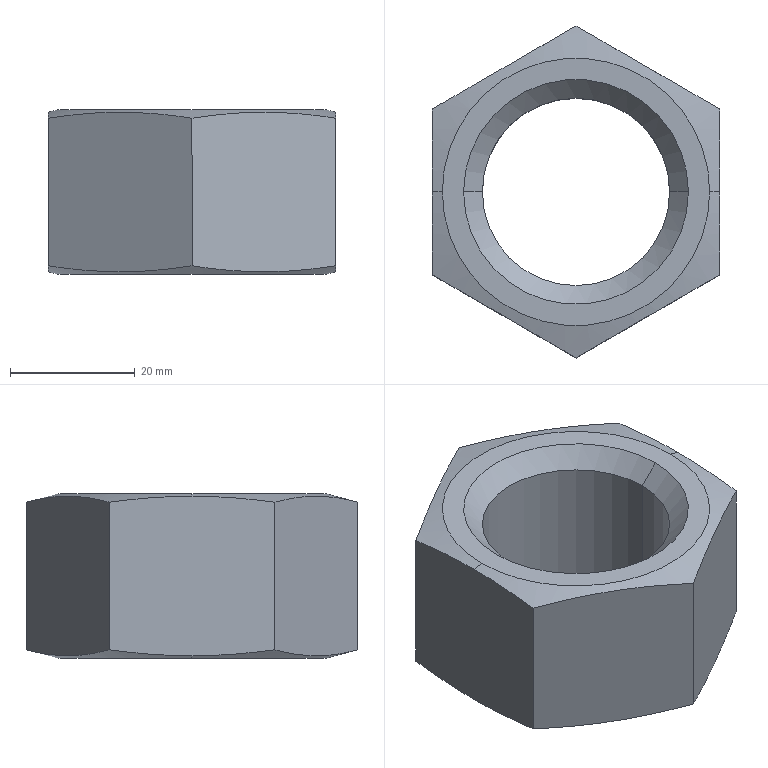Part | SolidWorks | features Chamfer 1, Extrusion 1, ICE 1, MirrorPattern 1, RevCutThin 1 | 1 solid | 18 faces | box 46 x 53.116 x 26.4 mm | volume 28471 mm3 | cone 8 | plane 8 | cylinder 2 | commonest cylinder face diameters 30 x2
STEP:
#1=CARTESIAN_POINT('',(-15.,0.,10.2));
#2=VERTEX_POINT('',#1);
#3=CARTESIAN_POINT('',(15.,0.,10.2));
#4=VERTEX_POINT('',#3);
#5=CARTESIAN_POINT('',(0.,0.,10.2));
#6=DIRECTION('',(0.,0.,1.));
#7=DIRECTION('',(1.,0.,0.));
#8=AXIS2_PLACEMENT_3D('',#5,#6,#7);
#9=CIRCLE('',#8,15.);
#10=EDGE_CURVE('',#2,#4,#9,.T.);
#11=ORIENTED_EDGE('',*,*,#10,.F.);
#12=CARTESIAN_POINT('',(-18.,0.,13.2));
#13=VERTEX_POINT('',#12);
#14=CARTESIAN_POINT('',(-15.,0.,10.2));
#15=DIRECTION('',(-0.7071,0.,0.7071));
#16=VECTOR('',#15,1000.);
#17=LINE('',#14,#16);
#18=EDGE_CURVE('',#2,#13,#17,.T.);
#19=ORIENTED_EDGE('',*,*,#18,.T.);
#20=CARTESIAN_POINT('',(18.,0.,13.2));
#21=VERTEX_POINT('',#20);
#22=CARTESIAN_POINT('',(0.,0.,13.2));
#23=DIRECTION('',(0.,0.,-1.));
#24=DIRECTION('',(1.,0.,0.));
#25=AXIS2_PLACEMENT_3D('',#22,#23,#24);
#26=CIRCLE('',#25,18.);
#27=EDGE_CURVE('',#21,#13,#26,.T.);
#28=ORIENTED_EDGE('',*,*,#27,.F.);
#29=CARTESIAN_POINT('',(15.,0.,10.2));
#30=DIRECTION('',(0.7071,0.,0.7071));
#31=VECTOR('',#30,1000.);
#32=LINE('',#29,#31);
#33=EDGE_CURVE('',#4,#21,#32,.T.);
#34=ORIENTED_EDGE('',*,*,#33,.F.);
#35=EDGE_LOOP('',(#11,#19,#28,#34));
#36=FACE_OUTER_BOUND('',#35,.T.);
#37=CARTESIAN_POINT('',(0.,0.,10.2));
#38=DIRECTION('',(0.,0.,1.));
#39=DIRECTION('',(1.,0.,0.));
#40=AXIS2_PLACEMENT_3D('',#37,#38,#39);
#41=CONICAL_SURFACE('',#40,15.,0.7854);
#42=ADVANCED_FACE('',(#36),#41,.F.);
#43=CARTESIAN_POINT('',(15.,0.,-10.2));
#44=VERTEX_POINT('',#43);
#45=CARTESIAN_POINT('',(-15.,0.,-10.2));
#46=VERTEX_POINT('',#45);
#47=CARTESIAN_POINT('',(0.,0.,-10.2));
#48=DIRECTION('',(0.,0.,-1.));
#49=DIRECTION('',(1.,0.,0.));
#50=AXIS2_PLACEMENT_3D('',#47,#48,#49);
#51=CIRCLE('',#50,15.);
#52=EDGE_CURVE('',#44,#46,#51,.T.);
#53=ORIENTED_EDGE('',*,*,#52,.F.);
#54=CARTESIAN_POINT('',(18.,0.,-13.2));
#55=VERTEX_POINT('',#54);
#56=CARTESIAN_POINT('',(18.,0.,-13.2));
#57=DIRECTION('',(0.7071,0.,-0.7071));
#58=VECTOR('',#57,1000.);
#59=LINE('',#56,#58);
#60=EDGE_CURVE('',#44,#55,#59,.T.);
#61=ORIENTED_EDGE('',*,*,#60,.T.);
#62=CARTESIAN_POINT('',(-18.,0.,-13.2));
#63=VERTEX_POINT('',#62);
#64=CARTESIAN_POINT('',(0.,0.,-13.2));
#65=DIRECTION('',(0.,0.,1.));
#66=DIRECTION('',(1.,0.,0.));
#67=AXIS2_PLACEMENT_3D('',#64,#65,#66);
#68=CIRCLE('',#67,18.);
#69=EDGE_CURVE('',#63,#55,#68,.T.);
#70=ORIENTED_EDGE('',*,*,#69,.F.);
#71=CARTESIAN_POINT('',(-18.,0.,-13.2));
#72=DIRECTION('',(-0.7071,0.,-0.7071));
#73=VECTOR('',#72,1000.);
#74=LINE('',#71,#73);
#75=EDGE_CURVE('',#46,#63,#74,.T.);
#76=ORIENTED_EDGE('',*,*,#75,.F.);
#77=EDGE_LOOP('',(#53,#61,#70,#76));
#78=FACE_OUTER_BOUND('',#77,.T.);
#79=CARTESIAN_POINT('',(0.,0.,-13.2));
#80=DIRECTION('',(0.,0.,-1.));
#81=DIRECTION('',(-1.,0.,0.));
#82=AXIS2_PLACEMENT_3D('',#79,#80,#81);
#83=CONICAL_SURFACE('',#82,18.,0.7854);
#84=ADVANCED_FACE('',(#78),#83,.F.);
#85=ORIENTED_EDGE('',*,*,#52,.T.);
#86=CARTESIAN_POINT('',(-15.,0.,-13.2));
#87=DIRECTION('',(0.,0.,1.));
#88=VECTOR('',#87,1000.);
#89=LINE('',#86,#88);
#90=EDGE_CURVE('',#46,#2,#89,.T.);
#91=ORIENTED_EDGE('',*,*,#90,.T.);
#92=ORIENTED_EDGE('',*,*,#10,.T.);
#93=CARTESIAN_POINT('',(15.,0.,-13.2));
#94=DIRECTION('',(0.,0.,1.));
#95=VECTOR('',#94,1000.);
#96=LINE('',#93,#95);
#97=EDGE_CURVE('',#44,#4,#96,.T.);
#98=ORIENTED_EDGE('',*,*,#97,.F.);
#99=EDGE_LOOP('',(#85,#91,#92,#98));
#100=FACE_OUTER_BOUND('',#99,.T.);
#101=CARTESIAN_POINT('',(0.,0.,-13.2));
#102=DIRECTION('',(0.,0.,1.));
#103=DIRECTION('',(1.,0.,0.));
#104=AXIS2_PLACEMENT_3D('',#101,#102,#103);
#105=CYLINDRICAL_SURFACE('',#104,15.);
#106=ADVANCED_FACE('',(#100),#105,.F.);
#107=CARTESIAN_POINT('',(21.4,0.,-13.2));
#108=VERTEX_POINT('',#107);
#109=CARTESIAN_POINT('',(-21.4,0.,-13.2));
#110=VERTEX_POINT('',#109);
#111=CARTESIAN_POINT('',(0.,0.,-13.2));
#112=DIRECTION('',(0.,0.,-1.));
#113=DIRECTION('',(-1.,0.,0.));
#114=AXIS2_PLACEMENT_3D('',#111,#112,#113);
#115=CIRCLE('',#114,21.4);
#116=EDGE_CURVE('',#108,#110,#115,.T.);
#117=ORIENTED_EDGE('',*,*,#116,.F.);
#118=CARTESIAN_POINT('',(23.,0.,-12.771));
#119=VERTEX_POINT('',#118);
#120=CARTESIAN_POINT('',(21.4,0.,-13.2));
#121=DIRECTION('',(0.9659,0.,0.2588));
#122=VECTOR('',#121,1000.);
#123=LINE('',#120,#122);
#124=EDGE_CURVE('',#108,#119,#123,.T.);
#125=ORIENTED_EDGE('',*,*,#124,.T.);
#126=CARTESIAN_POINT('',(23.,-13.279,-11.818));
#127=VERTEX_POINT('',#126);
#128=CARTESIAN_POINT('',(23.,-13.279,-11.818));
#129=CARTESIAN_POINT('',(23.,-11.073,-12.113));
#130=CARTESIAN_POINT('',(23.,-8.853,-12.355));
#131=CARTESIAN_POINT('',(23.,-4.423,-12.684));
#132=CARTESIAN_POINT('',(23.,-2.21,-12.771));
#133=CARTESIAN_POINT('',(23.,0.,-12.771));
#134=B_SPLINE_CURVE_WITH_KNOTS('',3,(#128,#129,#130,#131,#132,#133),.UNSPECIFIED.,.F.,.F.,(4,2,4),(0.02218,0.02885,0.03553),.UNSPECIFIED.);
#135=EDGE_CURVE('',#127,#119,#134,.T.);
#136=ORIENTED_EDGE('',*,*,#135,.F.);
#137=CARTESIAN_POINT('',(0.,-26.558,-11.818));
#138=VERTEX_POINT('',#137);
#139=CARTESIAN_POINT('',(0.,-26.558,-11.818));
#140=CARTESIAN_POINT('',(1.917,-25.452,-12.114));
#141=CARTESIAN_POINT('',(3.833,-24.345,-12.355));
#142=CARTESIAN_POINT('',(7.667,-22.132,-12.684));
#143=CARTESIAN_POINT('',(11.5,-19.919,-12.858));
#144=CARTESIAN_POINT('',(15.333,-17.705,-12.684));
#145=CARTESIAN_POINT('',(19.167,-15.492,-12.355));
#146=CARTESIAN_POINT('',(21.083,-14.386,-12.114));
#147=CARTESIAN_POINT('',(23.,-13.279,-11.818));
#148=B_SPLINE_CURVE_WITH_KNOTS('',3,(#139,#140,#141,#142,#143,#144,#145,#146,#147),.UNSPECIFIED.,.F.,.F.,(4,2,1,2,4),(0.000000231,0.00664,0.01328,0.01992,0.02656),.UNSPECIFIED.);
#149=EDGE_CURVE('',#138,#127,#148,.T.);
#150=ORIENTED_EDGE('',*,*,#149,.F.);
#151=CARTESIAN_POINT('',(-23.,-13.279,-11.818));
#152=VERTEX_POINT('',#151);
#153=CARTESIAN_POINT('',(-23.,-13.279,-11.818));
#154=CARTESIAN_POINT('',(-21.083,-14.386,-12.114));
#155=CARTESIAN_POINT('',(-19.167,-15.492,-12.355));
#156=CARTESIAN_POINT('',(-15.333,-17.705,-12.684));
#157=CARTESIAN_POINT('',(-11.5,-19.919,-12.858));
#158=CARTESIAN_POINT('',(-7.667,-22.132,-12.684));
#159=CARTESIAN_POINT('',(-3.833,-24.345,-12.355));
#160=CARTESIAN_POINT('',(-1.917,-25.452,-12.114));
#161=CARTESIAN_POINT('',(0.,-26.558,-11.818));
#162=B_SPLINE_CURVE_WITH_KNOTS('',3,(#153,#154,#155,#156,#157,#158,#159,#160,#161),.UNSPECIFIED.,.F.,.F.,(4,2,1,2,4),(0.000000231,0.00664,0.01328,0.01992,0.02656),.UNSPECIFIED.);
#163=EDGE_CURVE('',#152,#138,#162,.T.);
#164=ORIENTED_EDGE('',*,*,#163,.F.);
#165=CARTESIAN_POINT('',(-23.,0.,-12.771));
#166=VERTEX_POINT('',#165);
#167=CARTESIAN_POINT('',(-23.,0.,-12.771));
#168=CARTESIAN_POINT('',(-23.,-2.21,-12.771));
#169=CARTESIAN_POINT('',(-23.,-4.423,-12.684));
#170=CARTESIAN_POINT('',(-23.,-8.853,-12.355));
#171=CARTESIAN_POINT('',(-23.,-11.073,-12.113));
#172=CARTESIAN_POINT('',(-23.,-13.279,-11.818));
#173=B_SPLINE_CURVE_WITH_KNOTS('',3,(#167,#168,#169,#170,#171,#172),.UNSPECIFIED.,.F.,.F.,(4,2,4),(0.06399,0.07065,0.07731),.UNSPECIFIED.);
#174=EDGE_CURVE('',#166,#152,#173,.T.);
#175=ORIENTED_EDGE('',*,*,#174,.F.);
#176=CARTESIAN_POINT('',(-21.4,0.,-13.2));
#177=DIRECTION('',(-0.9659,0.,0.2588));
#178=VECTOR('',#177,1000.);
#179=LINE('',#176,#178);
#180=EDGE_CURVE('',#110,#166,#179,.T.);
#181=ORIENTED_EDGE('',*,*,#180,.F.);
#182=EDGE_LOOP('',(#117,#125,#136,#150,#164,#175,#181));
#183=FACE_OUTER_BOUND('',#182,.T.);
#184=CARTESIAN_POINT('',(0.,0.,-13.2));
#185=DIRECTION('',(0.,0.,1.));
#186=DIRECTION('',(-1.,0.,0.));
#187=AXIS2_PLACEMENT_3D('',#184,#185,#186);
#188=CONICAL_SURFACE('',#187,21.4,1.309);
#189=ADVANCED_FACE('',(#183),#188,.T.);
#190=CARTESIAN_POINT('',(-21.4,0.,13.2));
#191=VERTEX_POINT('',#190);
#192=CARTESIAN_POINT('',(21.4,0.,13.2));
#193=VERTEX_POINT('',#192);
#194=CARTESIAN_POINT('',(0.,0.,13.2));
#195=DIRECTION('',(0.,0.,-1.));
#196=DIRECTION('',(-1.,0.,0.));
#197=AXIS2_PLACEMENT_3D('',#194,#195,#196);
#198=CIRCLE('',#197,21.4);
#199=EDGE_CURVE('',#191,#193,#198,.T.);
#200=ORIENTED_EDGE('',*,*,#199,.T.);
#201=CARTESIAN_POINT('',(23.,0.,12.771));
#202=VERTEX_POINT('',#201);
#203=CARTESIAN_POINT('',(21.4,0.,13.2));
#204=DIRECTION('',(0.9659,0.,-0.2588));
#205=VECTOR('',#204,1000.);
#206=LINE('',#203,#205);
#207=EDGE_CURVE('',#193,#202,#206,.T.);
#208=ORIENTED_EDGE('',*,*,#207,.T.);
#209=CARTESIAN_POINT('',(23.,13.279,11.818));
#210=VERTEX_POINT('',#209);
#211=CARTESIAN_POINT('',(23.,13.279,11.818));
#212=CARTESIAN_POINT('',(23.,11.07,12.114));
#213=CARTESIAN_POINT('',(23.,8.859,12.355));
#214=CARTESIAN_POINT('',(23.,4.433,12.684));
#215=CARTESIAN_POINT('',(23.,2.218,12.771));
#216=CARTESIAN_POINT('',(23.,0.,12.771));
#217=B_SPLINE_CURVE_WITH_KNOTS('',3,(#211,#212,#213,#214,#215,#216),.UNSPECIFIED.,.F.,.F.,(4,2,4),(0.05062,0.0573,0.06399),.UNSPECIFIED.);
#218=EDGE_CURVE('',#210,#202,#217,.T.);
#219=ORIENTED_EDGE('',*,*,#218,.F.);
#220=CARTESIAN_POINT('',(0.,26.558,11.818));
#221=VERTEX_POINT('',#220);
#222=CARTESIAN_POINT('',(0.,26.558,11.818));
#223=CARTESIAN_POINT('',(1.917,25.452,12.114));
#224=CARTESIAN_POINT('',(3.833,24.345,12.355));
#225=CARTESIAN_POINT('',(7.667,22.132,12.684));
#226=CARTESIAN_POINT('',(11.5,19.919,12.858));
#227=CARTESIAN_POINT('',(15.333,17.705,12.684));
#228=CARTESIAN_POINT('',(19.167,15.492,12.355));
#229=CARTESIAN_POINT('',(21.083,14.386,12.114));
#230=CARTESIAN_POINT('',(23.,13.279,11.818));
#231=B_SPLINE_CURVE_WITH_KNOTS('',3,(#222,#223,#224,#225,#226,#227,#228,#229,#230),.UNSPECIFIED.,.F.,.F.,(4,2,1,2,4),(0.000000231,0.00664,0.01328,0.01992,0.02656),.UNSPECIFIED.);
#232=EDGE_CURVE('',#221,#210,#231,.T.);
#233=ORIENTED_EDGE('',*,*,#232,.F.);
#234=CARTESIAN_POINT('',(-23.,13.279,11.818));
#235=VERTEX_POINT('',#234);
#236=CARTESIAN_POINT('',(-23.,13.279,11.818));
#237=CARTESIAN_POINT('',(-21.083,14.386,12.114));
#238=CARTESIAN_POINT('',(-19.167,15.492,12.355));
#239=CARTESIAN_POINT('',(-15.333,17.705,12.684));
#240=CARTESIAN_POINT('',(-11.5,19.919,12.858));
#241=CARTESIAN_POINT('',(-7.667,22.132,12.684));
#242=CARTESIAN_POINT('',(-3.833,24.345,12.355));
#243=CARTESIAN_POINT('',(-1.917,25.452,12.114));
#244=CARTESIAN_POINT('',(0.,26.558,11.818));
#245=B_SPLINE_CURVE_WITH_KNOTS('',3,(#236,#237,#238,#239,#240,#241,#242,#243,#244),.UNSPECIFIED.,.F.,.F.,(4,2,1,2,4),(0.000000231,0.00664,0.01328,0.01992,0.02656),.UNSPECIFIED.);
#246=EDGE_CURVE('',#235,#221,#245,.T.);
#247=ORIENTED_EDGE('',*,*,#246,.F.);
#248=CARTESIAN_POINT('',(-23.,0.,12.771));
#249=VERTEX_POINT('',#248);
#250=CARTESIAN_POINT('',(-23.,0.,12.771));
#251=CARTESIAN_POINT('',(-23.,2.218,12.771));
#252=CARTESIAN_POINT('',(-23.,4.433,12.684));
#253=CARTESIAN_POINT('',(-23.,8.859,12.355));
#254=CARTESIAN_POINT('',(-23.,11.07,12.114));
#255=CARTESIAN_POINT('',(-23.,13.279,11.818));
#256=B_SPLINE_CURVE_WITH_KNOTS('',3,(#250,#251,#252,#253,#254,#255),.UNSPECIFIED.,.F.,.F.,(4,2,4),(0.03553,0.04222,0.04892),.UNSPECIFIED.);
#257=EDGE_CURVE('',#249,#235,#256,.T.);
#258=ORIENTED_EDGE('',*,*,#257,.F.);
#259=CARTESIAN_POINT('',(-21.4,0.,13.2));
#260=DIRECTION('',(-0.9659,0.,-0.2588));
#261=VECTOR('',#260,1000.);
#262=LINE('',#259,#261);
#263=EDGE_CURVE('',#191,#249,#262,.T.);
#264=ORIENTED_EDGE('',*,*,#263,.F.);
#265=EDGE_LOOP('',(#200,#208,#219,#233,#247,#258,#264));
#266=FACE_OUTER_BOUND('',#265,.T.);
#267=CARTESIAN_POINT('',(0.,0.,13.2));
#268=DIRECTION('',(0.,0.,-1.));
#269=DIRECTION('',(-1.,0.,0.));
#270=AXIS2_PLACEMENT_3D('',#267,#268,#269);
#271=CONICAL_SURFACE('',#270,21.4,1.309);
#272=ADVANCED_FACE('',(#266),#271,.T.);
#273=CARTESIAN_POINT('',(23.,-13.279,11.818));
#274=VERTEX_POINT('',#273);
#275=CARTESIAN_POINT('',(23.,-13.279,13.2));
#276=DIRECTION('',(0.,0.,-1.));
#277=VECTOR('',#276,1000.);
#278=LINE('',#275,#277);
#279=EDGE_CURVE('',#274,#127,#278,.T.);
#280=ORIENTED_EDGE('',*,*,#279,.T.);
#281=ORIENTED_EDGE('',*,*,#135,.T.);
#282=CARTESIAN_POINT('',(23.,13.279,-11.818));
#283=VERTEX_POINT('',#282);
#284=CARTESIAN_POINT('',(23.,0.,-12.771));
#285=CARTESIAN_POINT('',(23.,2.218,-12.771));
#286=CARTESIAN_POINT('',(23.,4.433,-12.684));
#287=CARTESIAN_POINT('',(23.,8.859,-12.355));
#288=CARTESIAN_POINT('',(23.,11.07,-12.114));
#289=CARTESIAN_POINT('',(23.,13.279,-11.818));
#290=B_SPLINE_CURVE_WITH_KNOTS('',3,(#284,#285,#286,#287,#288,#289),.UNSPECIFIED.,.F.,.F.,(4,2,4),(0.03553,0.04222,0.04892),.UNSPECIFIED.);
#291=EDGE_CURVE('',#119,#283,#290,.T.);
#292=ORIENTED_EDGE('',*,*,#291,.T.);
#293=CARTESIAN_POINT('',(23.,13.279,13.2));
#294=DIRECTION('',(0.,0.,-1.));
#295=VECTOR('',#294,1000.);
#296=LINE('',#293,#295);
#297=EDGE_CURVE('',#210,#283,#296,.T.);
#298=ORIENTED_EDGE('',*,*,#297,.F.);
#299=ORIENTED_EDGE('',*,*,#218,.T.);
#300=CARTESIAN_POINT('',(23.,0.,12.771));
#301=CARTESIAN_POINT('',(23.,-2.21,12.771));
#302=CARTESIAN_POINT('',(23.,-4.423,12.684));
#303=CARTESIAN_POINT('',(23.,-8.853,12.355));
#304=CARTESIAN_POINT('',(23.,-11.073,12.113));
#305=CARTESIAN_POINT('',(23.,-13.279,11.818));
#306=B_SPLINE_CURVE_WITH_KNOTS('',3,(#300,#301,#302,#303,#304,#305),.UNSPECIFIED.,.F.,.F.,(4,2,4),(0.06399,0.07065,0.07731),.UNSPECIFIED.);
#307=EDGE_CURVE('',#202,#274,#306,.T.);
#308=ORIENTED_EDGE('',*,*,#307,.T.);
#309=EDGE_LOOP('',(#280,#281,#292,#298,#299,#308));
#310=FACE_OUTER_BOUND('',#309,.T.);
#311=CARTESIAN_POINT('',(23.,-13.279,13.2));
#312=DIRECTION('',(-1.,0.,0.));
#313=DIRECTION('',(0.,-1.,0.));
#314=AXIS2_PLACEMENT_3D('',#311,#312,#313);
#315=PLANE('',#314);
#316=ADVANCED_FACE('',(#310),#315,.F.);
#317=ORIENTED_EDGE('',*,*,#297,.T.);
#318=CARTESIAN_POINT('',(0.,26.558,-11.818));
#319=VERTEX_POINT('',#318);
#320=CARTESIAN_POINT('',(23.,13.279,-11.818));
#321=CARTESIAN_POINT('',(21.083,14.386,-12.114));
#322=CARTESIAN_POINT('',(19.167,15.492,-12.355));
#323=CARTESIAN_POINT('',(15.333,17.705,-12.684));
#324=CARTESIAN_POINT('',(11.5,19.919,-12.858));
#325=CARTESIAN_POINT('',(7.667,22.132,-12.684));
#326=CARTESIAN_POINT('',(3.833,24.345,-12.355));
#327=CARTESIAN_POINT('',(1.917,25.452,-12.114));
#328=CARTESIAN_POINT('',(0.,26.558,-11.818));
#329=B_SPLINE_CURVE_WITH_KNOTS('',3,(#320,#321,#322,#323,#324,#325,#326,#327,#328),.UNSPECIFIED.,.F.,.F.,(4,2,1,2,4),(0.000000231,0.00664,0.01328,0.01992,0.02656),.UNSPECIFIED.);
#330=EDGE_CURVE('',#283,#319,#329,.T.);
#331=ORIENTED_EDGE('',*,*,#330,.T.);
#332=CARTESIAN_POINT('',(0.,26.558,13.2));
#333=DIRECTION('',(0.,0.,-1.));
#334=VECTOR('',#333,1000.);
#335=LINE('',#332,#334);
#336=EDGE_CURVE('',#221,#319,#335,.T.);
#337=ORIENTED_EDGE('',*,*,#336,.F.);
#338=ORIENTED_EDGE('',*,*,#232,.T.);
#339=EDGE_LOOP('',(#317,#331,#337,#338));
#340=FACE_OUTER_BOUND('',#339,.T.);
#341=CARTESIAN_POINT('',(23.,13.279,13.2));
#342=DIRECTION('',(-0.5,-0.866,0.));
#343=DIRECTION('',(0.866,-0.5,0.));
#344=AXIS2_PLACEMENT_3D('',#341,#342,#343);
#345=PLANE('',#344);
#346=ADVANCED_FACE('',(#340),#345,.F.);
#347=ORIENTED_EDGE('',*,*,#336,.T.);
#348=CARTESIAN_POINT('',(-23.,13.279,-11.818));
#349=VERTEX_POINT('',#348);
#350=CARTESIAN_POINT('',(0.,26.558,-11.818));
#351=CARTESIAN_POINT('',(-1.917,25.452,-12.114));
#352=CARTESIAN_POINT('',(-3.833,24.345,-12.355));
#353=CARTESIAN_POINT('',(-7.667,22.132,-12.684));
#354=CARTESIAN_POINT('',(-11.5,19.919,-12.858));
#355=CARTESIAN_POINT('',(-15.333,17.705,-12.684));
#356=CARTESIAN_POINT('',(-19.167,15.492,-12.355));
#357=CARTESIAN_POINT('',(-21.083,14.386,-12.114));
#358=CARTESIAN_POINT('',(-23.,13.279,-11.818));
#359=B_SPLINE_CURVE_WITH_KNOTS('',3,(#350,#351,#352,#353,#354,#355,#356,#357,#358),.UNSPECIFIED.,.F.,.F.,(4,2,1,2,4),(0.000000231,0.00664,0.01328,0.01992,0.02656),.UNSPECIFIED.);
#360=EDGE_CURVE('',#319,#349,#359,.T.);
#361=ORIENTED_EDGE('',*,*,#360,.T.);
#362=CARTESIAN_POINT('',(-23.,13.279,13.2));
#363=DIRECTION('',(0.,0.,-1.));
#364=VECTOR('',#363,1000.);
#365=LINE('',#362,#364);
#366=EDGE_CURVE('',#235,#349,#365,.T.);
#367=ORIENTED_EDGE('',*,*,#366,.F.);
#368=ORIENTED_EDGE('',*,*,#246,.T.);
#369=EDGE_LOOP('',(#347,#361,#367,#368));
#370=FACE_OUTER_BOUND('',#369,.T.);
#371=CARTESIAN_POINT('',(0.,26.558,13.2));
#372=DIRECTION('',(0.5,-0.866,0.));
#373=DIRECTION('',(0.866,0.5,0.));
#374=AXIS2_PLACEMENT_3D('',#371,#372,#373);
#375=PLANE('',#374);
#376=ADVANCED_FACE('',(#370),#375,.F.);
#377=ORIENTED_EDGE('',*,*,#366,.T.);
#378=CARTESIAN_POINT('',(-23.,13.279,-11.818));
#379=CARTESIAN_POINT('',(-23.,11.07,-12.114));
#380=CARTESIAN_POINT('',(-23.,8.859,-12.355));
#381=CARTESIAN_POINT('',(-23.,4.433,-12.684));
#382=CARTESIAN_POINT('',(-23.,2.218,-12.771));
#383=CARTESIAN_POINT('',(-23.,0.,-12.771));
#384=B_SPLINE_CURVE_WITH_KNOTS('',3,(#378,#379,#380,#381,#382,#383),.UNSPECIFIED.,.F.,.F.,(4,2,4),(0.05062,0.0573,0.06399),.UNSPECIFIED.);
#385=EDGE_CURVE('',#349,#166,#384,.T.);
#386=ORIENTED_EDGE('',*,*,#385,.T.);
#387=ORIENTED_EDGE('',*,*,#174,.T.);
#388=CARTESIAN_POINT('',(-23.,-13.279,11.818));
#389=VERTEX_POINT('',#388);
#390=CARTESIAN_POINT('',(-23.,-13.279,13.2));
#391=DIRECTION('',(0.,0.,-1.));
#392=VECTOR('',#391,1000.);
#393=LINE('',#390,#392);
#394=EDGE_CURVE('',#389,#152,#393,.T.);
#395=ORIENTED_EDGE('',*,*,#394,.F.);
#396=CARTESIAN_POINT('',(-23.,-13.279,11.818));
#397=CARTESIAN_POINT('',(-23.,-11.073,12.113));
#398=CARTESIAN_POINT('',(-23.,-8.853,12.355));
#399=CARTESIAN_POINT('',(-23.,-4.423,12.684));
#400=CARTESIAN_POINT('',(-23.,-2.21,12.771));
#401=CARTESIAN_POINT('',(-23.,0.,12.771));
#402=B_SPLINE_CURVE_WITH_KNOTS('',3,(#396,#397,#398,#399,#400,#401),.UNSPECIFIED.,.F.,.F.,(4,2,4),(0.02218,0.02885,0.03553),.UNSPECIFIED.);
#403=EDGE_CURVE('',#389,#249,#402,.T.);
#404=ORIENTED_EDGE('',*,*,#403,.T.);
#405=ORIENTED_EDGE('',*,*,#257,.T.);
#406=EDGE_LOOP('',(#377,#386,#387,#395,#404,#405));
#407=FACE_OUTER_BOUND('',#406,.T.);
#408=CARTESIAN_POINT('',(-23.,13.279,13.2));
#409=DIRECTION('',(1.,0.,0.));
#410=DIRECTION('',(0.,1.,0.));
#411=AXIS2_PLACEMENT_3D('',#408,#409,#410);
#412=PLANE('',#411);
#413=ADVANCED_FACE('',(#407),#412,.F.);
#414=ORIENTED_EDGE('',*,*,#394,.T.);
#415=ORIENTED_EDGE('',*,*,#163,.T.);
#416=CARTESIAN_POINT('',(0.,-26.558,11.818));
#417=VERTEX_POINT('',#416);
#418=CARTESIAN_POINT('',(0.,-26.558,13.2));
#419=DIRECTION('',(0.,0.,-1.));
#420=VECTOR('',#419,1000.);
#421=LINE('',#418,#420);
#422=EDGE_CURVE('',#417,#138,#421,.T.);
#423=ORIENTED_EDGE('',*,*,#422,.F.);
#424=CARTESIAN_POINT('',(0.,-26.558,11.818));
#425=CARTESIAN_POINT('',(-1.917,-25.452,12.114));
#426=CARTESIAN_POINT('',(-3.833,-24.345,12.355));
#427=CARTESIAN_POINT('',(-7.667,-22.132,12.684));
#428=CARTESIAN_POINT('',(-11.5,-19.919,12.858));
#429=CARTESIAN_POINT('',(-15.333,-17.705,12.684));
#430=CARTESIAN_POINT('',(-19.167,-15.492,12.355));
#431=CARTESIAN_POINT('',(-21.083,-14.386,12.114));
#432=CARTESIAN_POINT('',(-23.,-13.279,11.818));
#433=B_SPLINE_CURVE_WITH_KNOTS('',3,(#424,#425,#426,#427,#428,#429,#430,#431,#432),.UNSPECIFIED.,.F.,.F.,(4,2,1,2,4),(0.000000231,0.00664,0.01328,0.01992,0.02656),.UNSPECIFIED.);
#434=EDGE_CURVE('',#417,#389,#433,.T.);
#435=ORIENTED_EDGE('',*,*,#434,.T.);
#436=EDGE_LOOP('',(#414,#415,#423,#435));
#437=FACE_OUTER_BOUND('',#436,.T.);
#438=CARTESIAN_POINT('',(-23.,-13.279,13.2));
#439=DIRECTION('',(0.5,0.866,0.));
#440=DIRECTION('',(-0.866,0.5,0.));
#441=AXIS2_PLACEMENT_3D('',#438,#439,#440);
#442=PLANE('',#441);
#443=ADVANCED_FACE('',(#437),#442,.F.);
#444=ORIENTED_EDGE('',*,*,#422,.T.);
#445=ORIENTED_EDGE('',*,*,#149,.T.);
#446=ORIENTED_EDGE('',*,*,#279,.F.);
#447=CARTESIAN_POINT('',(23.,-13.279,11.818));
#448=CARTESIAN_POINT('',(21.083,-14.386,12.114));
#449=CARTESIAN_POINT('',(19.167,-15.492,12.355));
#450=CARTESIAN_POINT('',(15.333,-17.705,12.684));
#451=CARTESIAN_POINT('',(11.5,-19.919,12.858));
#452=CARTESIAN_POINT('',(7.667,-22.132,12.684));
#453=CARTESIAN_POINT('',(3.833,-24.345,12.355));
#454=CARTESIAN_POINT('',(1.917,-25.452,12.114));
#455=CARTESIAN_POINT('',(0.,-26.558,11.818));
#456=B_SPLINE_CURVE_WITH_KNOTS('',3,(#447,#448,#449,#450,#451,#452,#453,#454,#455),.UNSPECIFIED.,.F.,.F.,(4,2,1,2,4),(0.000000231,0.00664,0.01328,0.01992,0.02656),.UNSPECIFIED.);
#457=EDGE_CURVE('',#274,#417,#456,.T.);
#458=ORIENTED_EDGE('',*,*,#457,.T.);
#459=EDGE_LOOP('',(#444,#445,#446,#458));
#460=FACE_OUTER_BOUND('',#459,.T.);
#461=CARTESIAN_POINT('',(0.,-26.558,13.2));
#462=DIRECTION('',(-0.5,0.866,0.));
#463=DIRECTION('',(-0.866,-0.5,0.));
#464=AXIS2_PLACEMENT_3D('',#461,#462,#463);
#465=PLANE('',#464);
#466=ADVANCED_FACE('',(#460),#465,.F.);
#467=ORIENTED_EDGE('',*,*,#207,.F.);
#468=CARTESIAN_POINT('',(0.,0.,13.2));
#469=DIRECTION('',(0.,0.,-1.));
#470=DIRECTION('',(-1.,0.,0.));
#471=AXIS2_PLACEMENT_3D('',#468,#469,#470);
#472=CIRCLE('',#471,21.4);
#473=EDGE_CURVE('',#193,#191,#472,.T.);
#474=ORIENTED_EDGE('',*,*,#473,.T.);
#475=ORIENTED_EDGE('',*,*,#263,.T.);
#476=ORIENTED_EDGE('',*,*,#403,.F.);
#477=ORIENTED_EDGE('',*,*,#434,.F.);
#478=ORIENTED_EDGE('',*,*,#457,.F.);
#479=ORIENTED_EDGE('',*,*,#307,.F.);
#480=EDGE_LOOP('',(#467,#474,#475,#476,#477,#478,#479));
#481=FACE_OUTER_BOUND('',#480,.T.);
#482=CARTESIAN_POINT('',(0.,0.,13.2));
#483=DIRECTION('',(0.,0.,-1.));
#484=DIRECTION('',(-1.,0.,0.));
#485=AXIS2_PLACEMENT_3D('',#482,#483,#484);
#486=CONICAL_SURFACE('',#485,21.4,1.309);
#487=ADVANCED_FACE('',(#481),#486,.T.);
#488=ORIENTED_EDGE('',*,*,#27,.T.);
#489=CARTESIAN_POINT('',(0.,0.,13.2));
#490=DIRECTION('',(0.,0.,-1.));
#491=DIRECTION('',(1.,0.,0.));
#492=AXIS2_PLACEMENT_3D('',#489,#490,#491);
#493=CIRCLE('',#492,18.);
#494=EDGE_CURVE('',#13,#21,#493,.T.);
#495=ORIENTED_EDGE('',*,*,#494,.T.);
#496=EDGE_LOOP('',(#488,#495));
#497=FACE_BOUND('',#496,.T.);
#498=ORIENTED_EDGE('',*,*,#199,.F.);
#499=ORIENTED_EDGE('',*,*,#473,.F.);
#500=EDGE_LOOP('',(#498,#499));
#501=FACE_OUTER_BOUND('',#500,.T.);
#502=CARTESIAN_POINT('',(0.,0.,13.2));
#503=DIRECTION('',(0.,0.,1.));
#504=DIRECTION('',(1.,0.,0.));
#505=AXIS2_PLACEMENT_3D('',#502,#503,#504);
#506=PLANE('',#505);
#507=ADVANCED_FACE('',(#497,#501),#506,.T.);
#508=ORIENTED_EDGE('',*,*,#124,.F.);
#509=CARTESIAN_POINT('',(0.,0.,-13.2));
#510=DIRECTION('',(0.,0.,-1.));
#511=DIRECTION('',(-1.,0.,0.));
#512=AXIS2_PLACEMENT_3D('',#509,#510,#511);
#513=CIRCLE('',#512,21.4);
#514=EDGE_CURVE('',#110,#108,#513,.T.);
#515=ORIENTED_EDGE('',*,*,#514,.F.);
#516=ORIENTED_EDGE('',*,*,#180,.T.);
#517=ORIENTED_EDGE('',*,*,#385,.F.);
#518=ORIENTED_EDGE('',*,*,#360,.F.);
#519=ORIENTED_EDGE('',*,*,#330,.F.);
#520=ORIENTED_EDGE('',*,*,#291,.F.);
#521=EDGE_LOOP('',(#508,#515,#516,#517,#518,#519,#520));
#522=FACE_OUTER_BOUND('',#521,.T.);
#523=CARTESIAN_POINT('',(0.,0.,-13.2));
#524=DIRECTION('',(0.,0.,1.));
#525=DIRECTION('',(-1.,0.,0.));
#526=AXIS2_PLACEMENT_3D('',#523,#524,#525);
#527=CONICAL_SURFACE('',#526,21.4,1.309);
#528=ADVANCED_FACE('',(#522),#527,.T.);
#529=ORIENTED_EDGE('',*,*,#69,.T.);
#530=CARTESIAN_POINT('',(0.,0.,-13.2));
#531=DIRECTION('',(0.,0.,1.));
#532=DIRECTION('',(1.,0.,0.));
#533=AXIS2_PLACEMENT_3D('',#530,#531,#532);
#534=CIRCLE('',#533,18.);
#535=EDGE_CURVE('',#55,#63,#534,.T.);
#536=ORIENTED_EDGE('',*,*,#535,.T.);
#537=EDGE_LOOP('',(#529,#536));
#538=FACE_BOUND('',#537,.T.);
#539=ORIENTED_EDGE('',*,*,#514,.T.);
#540=ORIENTED_EDGE('',*,*,#116,.T.);
#541=EDGE_LOOP('',(#539,#540));
#542=FACE_OUTER_BOUND('',#541,.T.);
#543=CARTESIAN_POINT('',(0.,0.,-13.2));
#544=DIRECTION('',(0.,0.,1.));
#545=DIRECTION('',(1.,0.,0.));
#546=AXIS2_PLACEMENT_3D('',#543,#544,#545);
#547=PLANE('',#546);
#548=ADVANCED_FACE('',(#538,#542),#547,.F.);
#549=ORIENTED_EDGE('',*,*,#90,.F.);
#550=CARTESIAN_POINT('',(0.,0.,-10.2));
#551=DIRECTION('',(0.,0.,-1.));
#552=DIRECTION('',(1.,0.,0.));
#553=AXIS2_PLACEMENT_3D('',#550,#551,#552);
#554=CIRCLE('',#553,15.);
#555=EDGE_CURVE('',#46,#44,#554,.T.);
#556=ORIENTED_EDGE('',*,*,#555,.T.);
#557=ORIENTED_EDGE('',*,*,#97,.T.);
#558=CARTESIAN_POINT('',(0.,0.,10.2));
#559=DIRECTION('',(0.,0.,1.));
#560=DIRECTION('',(1.,0.,0.));
#561=AXIS2_PLACEMENT_3D('',#558,#559,#560);
#562=CIRCLE('',#561,15.);
#563=EDGE_CURVE('',#4,#2,#562,.T.);
#564=ORIENTED_EDGE('',*,*,#563,.T.);
#565=EDGE_LOOP('',(#549,#556,#557,#564));
#566=FACE_OUTER_BOUND('',#565,.T.);
#567=CARTESIAN_POINT('',(0.,0.,-13.2));
#568=DIRECTION('',(0.,0.,1.));
#569=DIRECTION('',(1.,0.,0.));
#570=AXIS2_PLACEMENT_3D('',#567,#568,#569);
#571=CYLINDRICAL_SURFACE('',#570,15.);
#572=ADVANCED_FACE('',(#566),#571,.F.);
#573=ORIENTED_EDGE('',*,*,#60,.F.);
#574=ORIENTED_EDGE('',*,*,#555,.F.);
#575=ORIENTED_EDGE('',*,*,#75,.T.);
#576=ORIENTED_EDGE('',*,*,#535,.F.);
#577=EDGE_LOOP('',(#573,#574,#575,#576));
#578=FACE_OUTER_BOUND('',#577,.T.);
#579=CARTESIAN_POINT('',(0.,0.,-13.2));
#580=DIRECTION('',(0.,0.,-1.));
#581=DIRECTION('',(-1.,0.,0.));
#582=AXIS2_PLACEMENT_3D('',#579,#580,#581);
#583=CONICAL_SURFACE('',#582,18.,0.7854);
#584=ADVANCED_FACE('',(#578),#583,.F.);
#585=ORIENTED_EDGE('',*,*,#18,.F.);
#586=ORIENTED_EDGE('',*,*,#563,.F.);
#587=ORIENTED_EDGE('',*,*,#33,.T.);
#588=ORIENTED_EDGE('',*,*,#494,.F.);
#589=EDGE_LOOP('',(#585,#586,#587,#588));
#590=FACE_OUTER_BOUND('',#589,.T.);
#591=CARTESIAN_POINT('',(0.,0.,10.2));
#592=DIRECTION('',(0.,0.,1.));
#593=DIRECTION('',(1.,0.,0.));
#594=AXIS2_PLACEMENT_3D('',#591,#592,#593);
#595=CONICAL_SURFACE('',#594,15.,0.7854);
#596=ADVANCED_FACE('',(#590),#595,.F.);
#597=CLOSED_SHELL('',(#42,#84,#106,#189,#272,#316,#346,#376,#413,#443,#466,#487,#507,#528,#548,#572,#584,#596));
#598=MANIFOLD_SOLID_BREP('',#597);
#599=CARTESIAN_POINT('',(0.,0.,0.));
#600=DIRECTION('',(0.,0.,1.));
#601=DIRECTION('',(1.,0.,0.));
#602=AXIS2_PLACEMENT_3D('',#599,#600,#601);
#603=(LENGTH_UNIT()NAMED_UNIT(*)SI_UNIT(.MILLI.,.METRE.));
#604=UNCERTAINTY_MEASURE_WITH_UNIT(LENGTH_MEASURE(0.00001),#603,'','');
#605=(NAMED_UNIT(*)PLANE_ANGLE_UNIT()SI_UNIT($,.RADIAN.));
#606=(NAMED_UNIT(*)SI_UNIT($,.STERADIAN.)SOLID_ANGLE_UNIT());
#607=(GEOMETRIC_REPRESENTATION_CONTEXT(3)GLOBAL_UNCERTAINTY_ASSIGNED_CONTEXT((#604))GLOBAL_UNIT_ASSIGNED_CONTEXT((#603,#605,#606))REPRESENTATION_CONTEXT('',''));
#608=ADVANCED_BREP_SHAPE_REPRESENTATION('',(#598,#602),#607);